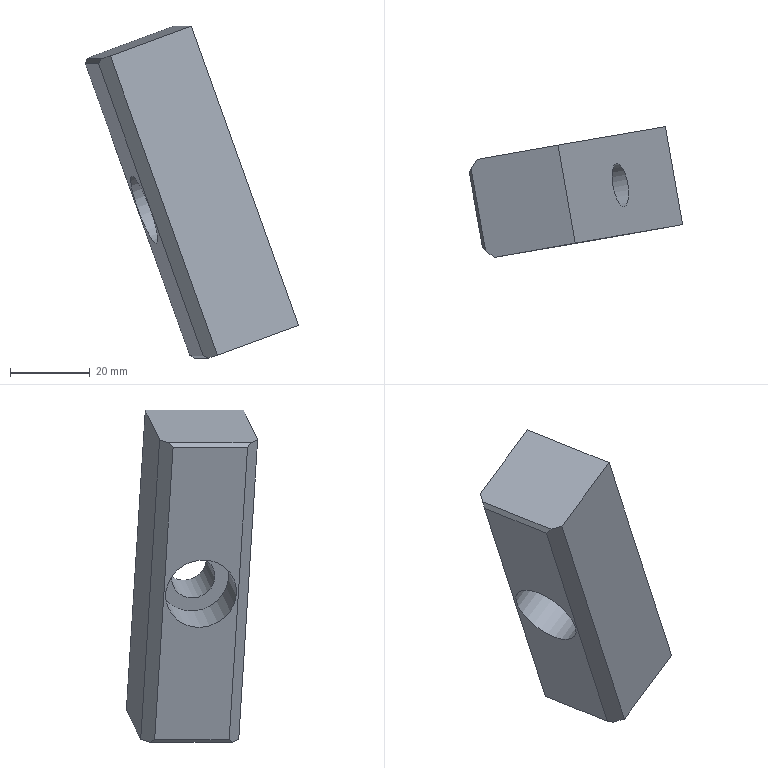Part | NX | features solid 2 | 1 solid | 13 faces | box 53.565 x 32.961 x 83.384 mm | volume 44971 mm3 | plane 11 | cylinder 2 | commonest cylinder face diameters 11 x1 18 x1
STEP:
#1=CARTESIAN_POINT('',(896.041,-33.81,-58.145));
#2=VERTEX_POINT('',#1);
#3=CARTESIAN_POINT('',(875.682,-37.399,-65.669));
#4=VERTEX_POINT('',#3);
#5=CARTESIAN_POINT('',(896.041,-33.81,-58.145));
#6=DIRECTION('',(-0.9254,-0.1632,-0.342));
#7=VECTOR('',#6,1000.);
#8=LINE('',#5,#7);
#9=EDGE_CURVE('',#2,#4,#8,.T.);
#10=ORIENTED_EDGE('',*,*,#9,.T.);
#11=CARTESIAN_POINT('',(902.628,-32.648,-140.845));
#12=VERTEX_POINT('',#11);
#13=CARTESIAN_POINT('',(875.682,-37.399,-65.669));
#14=DIRECTION('',(0.3368,0.05939,-0.9397));
#15=VECTOR('',#14,1000.);
#16=LINE('',#13,#15);
#17=EDGE_CURVE('',#4,#12,#16,.T.);
#18=ORIENTED_EDGE('',*,*,#17,.T.);
#19=CARTESIAN_POINT('',(922.987,-29.058,-133.32));
#20=VERTEX_POINT('',#19);
#21=CARTESIAN_POINT('',(922.987,-29.058,-133.32));
#22=DIRECTION('',(-0.9254,-0.1632,-0.342));
#23=VECTOR('',#22,1000.);
#24=LINE('',#21,#23);
#25=EDGE_CURVE('',#20,#12,#24,.T.);
#26=ORIENTED_EDGE('',*,*,#25,.F.);
#27=CARTESIAN_POINT('',(896.041,-33.81,-58.145));
#28=DIRECTION('',(0.3368,0.05939,-0.9397));
#29=VECTOR('',#28,1000.);
#30=LINE('',#27,#29);
#31=EDGE_CURVE('',#2,#20,#30,.T.);
#32=ORIENTED_EDGE('',*,*,#31,.F.);
#33=EDGE_LOOP('',(#10,#18,#26,#32));
#34=FACE_BOUND('',#33,.T.);
#35=CARTESIAN_POINT('',(896.041,-33.81,-58.145));
#36=DIRECTION('',(0.1736,-0.9848,0.));
#37=DIRECTION('',(-0.9254,-0.1632,-0.342));
#38=AXIS2_PLACEMENT_3D('',#35,#36,#37);
#39=PLANE('',#38);
#40=ADVANCED_FACE('',(#34),#39,.T.);
#41=CARTESIAN_POINT('',(887.328,-23.203,-112.725));
#42=VERTEX_POINT('',#41);
#43=CARTESIAN_POINT('',(884.208,-23.203,-104.283));
#44=DIRECTION('',(0.9254,0.1632,0.342));
#45=DIRECTION('',(0.3467,0.,-0.938));
#46=AXIS2_PLACEMENT_3D('',#43,#44,#45);
#47=CIRCLE('',#46,9.);
#48=EDGE_CURVE('',#42,#42,#47,.T.);
#49=ORIENTED_EDGE('',*,*,#48,.T.);
#50=EDGE_LOOP('',(#49));
#51=FACE_BOUND('',#50,.T.);
#52=CARTESIAN_POINT('',(898.994,-30.243,-140.931));
#53=VERTEX_POINT('',#52);
#54=CARTESIAN_POINT('',(872.721,-34.875,-67.635));
#55=VERTEX_POINT('',#54);
#56=CARTESIAN_POINT('',(872.385,-34.934,-66.695));
#57=DIRECTION('',(-0.3368,-0.05939,0.9397));
#58=VECTOR('',#57,1000.);
#59=LINE('',#56,#58);
#60=EDGE_CURVE('',#53,#55,#59,.T.);
#61=ORIENTED_EDGE('',*,*,#60,.T.);
#62=CARTESIAN_POINT('',(869.422,-16.164,-67.635));
#63=VERTEX_POINT('',#62);
#64=CARTESIAN_POINT('',(868.814,-12.717,-67.635));
#65=DIRECTION('',(-0.1736,0.9848,0.));
#66=VECTOR('',#65,1000.);
#67=LINE('',#64,#66);
#68=EDGE_CURVE('',#55,#63,#67,.T.);
#69=ORIENTED_EDGE('',*,*,#68,.T.);
#70=CARTESIAN_POINT('',(895.694,-11.531,-140.931));
#71=VERTEX_POINT('',#70);
#72=CARTESIAN_POINT('',(869.085,-16.223,-66.695));
#73=DIRECTION('',(0.3368,0.05939,-0.9397));
#74=VECTOR('',#73,1000.);
#75=LINE('',#72,#74);
#76=EDGE_CURVE('',#63,#71,#75,.T.);
#77=ORIENTED_EDGE('',*,*,#76,.T.);
#78=CARTESIAN_POINT('',(900.122,-36.644,-140.931));
#79=DIRECTION('',(0.1736,-0.9848,0.));
#80=VECTOR('',#79,1000.);
#81=LINE('',#78,#80);
#82=EDGE_CURVE('',#71,#53,#81,.T.);
#83=ORIENTED_EDGE('',*,*,#82,.T.);
#84=EDGE_LOOP('',(#61,#69,#77,#83));
#85=FACE_BOUND('',#84,.T.);
#86=CARTESIAN_POINT('',(873.513,-41.336,-66.695));
#87=DIRECTION('',(-0.9254,-0.1632,-0.342));
#88=DIRECTION('',(-0.1736,0.9848,0.));
#89=AXIS2_PLACEMENT_3D('',#86,#87,#88);
#90=PLANE('',#89);
#91=ADVANCED_FACE('',(#51,#85),#90,.T.);
#92=CARTESIAN_POINT('',(918.646,-4.438,-133.32));
#93=VERTEX_POINT('',#92);
#94=CARTESIAN_POINT('',(898.286,-8.028,-140.845));
#95=VERTEX_POINT('',#94);
#96=CARTESIAN_POINT('',(918.646,-4.438,-133.32));
#97=DIRECTION('',(0.9254,0.1632,0.342));
#98=VECTOR('',#97,1000.);
#99=LINE('',#96,#98);
#100=EDGE_CURVE('',#93,#95,#99,.F.);
#101=ORIENTED_EDGE('',*,*,#100,.T.);
#102=CARTESIAN_POINT('',(871.341,-12.779,-65.669));
#103=VERTEX_POINT('',#102);
#104=CARTESIAN_POINT('',(871.341,-12.779,-65.669));
#105=DIRECTION('',(0.3368,0.05939,-0.9397));
#106=VECTOR('',#105,1000.);
#107=LINE('',#104,#106);
#108=EDGE_CURVE('',#95,#103,#107,.F.);
#109=ORIENTED_EDGE('',*,*,#108,.T.);
#110=CARTESIAN_POINT('',(891.7,-9.189,-58.145));
#111=VERTEX_POINT('',#110);
#112=CARTESIAN_POINT('',(891.7,-9.189,-58.145));
#113=DIRECTION('',(0.9254,0.1632,0.342));
#114=VECTOR('',#113,1000.);
#115=LINE('',#112,#114);
#116=EDGE_CURVE('',#111,#103,#115,.F.);
#117=ORIENTED_EDGE('',*,*,#116,.F.);
#118=CARTESIAN_POINT('',(891.7,-9.189,-58.145));
#119=DIRECTION('',(0.3368,0.05939,-0.9397));
#120=VECTOR('',#119,1000.);
#121=LINE('',#118,#120);
#122=EDGE_CURVE('',#111,#93,#121,.T.);
#123=ORIENTED_EDGE('',*,*,#122,.T.);
#124=EDGE_LOOP('',(#101,#109,#117,#123));
#125=FACE_BOUND('',#124,.T.);
#126=CARTESIAN_POINT('',(891.7,-9.189,-58.145));
#127=DIRECTION('',(0.1736,-0.9848,0.));
#128=DIRECTION('',(-0.9254,-0.1632,-0.342));
#129=AXIS2_PLACEMENT_3D('',#126,#127,#128);
#130=PLANE('',#129);
#131=ADVANCED_FACE('',(#125),#130,.F.);
#132=CARTESIAN_POINT('',(905.437,-19.124,-90.574));
#133=VERTEX_POINT('',#132);
#134=CARTESIAN_POINT('',(907.343,-19.124,-95.733));
#135=DIRECTION('',(-0.9254,-0.1632,-0.342));
#136=DIRECTION('',(-0.3467,0.,0.938));
#137=AXIS2_PLACEMENT_3D('',#134,#135,#136);
#138=CIRCLE('',#137,5.5);
#139=EDGE_CURVE('',#133,#133,#138,.F.);
#140=ORIENTED_EDGE('',*,*,#139,.F.);
#141=EDGE_LOOP('',(#140));
#142=FACE_BOUND('',#141,.T.);
#143=CARTESIAN_POINT('',(896.649,-37.256,-58.145));
#144=DIRECTION('',(-0.1736,0.9848,0.));
#145=VECTOR('',#144,1000.);
#146=LINE('',#143,#145);
#147=EDGE_CURVE('',#2,#111,#146,.T.);
#148=ORIENTED_EDGE('',*,*,#147,.F.);
#149=ORIENTED_EDGE('',*,*,#31,.T.);
#150=CARTESIAN_POINT('',(923.595,-32.505,-133.32));
#151=DIRECTION('',(-0.1736,0.9848,0.));
#152=VECTOR('',#151,1000.);
#153=LINE('',#150,#152);
#154=EDGE_CURVE('',#20,#93,#153,.T.);
#155=ORIENTED_EDGE('',*,*,#154,.T.);
#156=ORIENTED_EDGE('',*,*,#122,.F.);
#157=EDGE_LOOP('',(#148,#149,#155,#156));
#158=FACE_BOUND('',#157,.T.);
#159=CARTESIAN_POINT('',(896.649,-37.256,-58.145));
#160=DIRECTION('',(-0.9254,-0.1632,-0.342));
#161=DIRECTION('',(-0.1736,0.9848,0.));
#162=AXIS2_PLACEMENT_3D('',#159,#160,#161);
#163=PLANE('',#162);
#164=ADVANCED_FACE('',(#142,#158),#163,.F.);
#165=CARTESIAN_POINT('',(900.43,-31.005,-141.529));
#166=VERTEX_POINT('',#165);
#167=CARTESIAN_POINT('',(917.465,-43.74,-136.228));
#168=DIRECTION('',(0.7772,-0.581,0.2418));
#169=VECTOR('',#168,1000.);
#170=LINE('',#167,#169);
#171=EDGE_CURVE('',#12,#166,#170,.F.);
#172=ORIENTED_EDGE('',*,*,#171,.T.);
#173=CARTESIAN_POINT('',(896.783,-10.324,-141.529));
#174=VERTEX_POINT('',#173);
#175=CARTESIAN_POINT('',(901.385,-36.421,-141.529));
#176=DIRECTION('',(-0.1736,0.9848,0.));
#177=VECTOR('',#176,1000.);
#178=LINE('',#175,#177);
#179=EDGE_CURVE('',#166,#174,#178,.T.);
#180=ORIENTED_EDGE('',*,*,#179,.T.);
#181=CARTESIAN_POINT('',(896.407,-10.898,-141.7));
#182=DIRECTION('',(0.5316,0.8117,0.2418));
#183=VECTOR('',#182,1000.);
#184=LINE('',#181,#183);
#185=EDGE_CURVE('',#174,#95,#184,.T.);
#186=ORIENTED_EDGE('',*,*,#185,.T.);
#187=ORIENTED_EDGE('',*,*,#100,.F.);
#188=ORIENTED_EDGE('',*,*,#154,.F.);
#189=ORIENTED_EDGE('',*,*,#25,.T.);
#190=EDGE_LOOP('',(#172,#180,#186,#187,#188,#189));
#191=FACE_BOUND('',#190,.T.);
#192=CARTESIAN_POINT('',(923.595,-32.505,-133.32));
#193=DIRECTION('',(0.3368,0.05939,-0.9397));
#194=DIRECTION('',(-0.9414,0.,-0.3374));
#195=AXIS2_PLACEMENT_3D('',#192,#193,#194);
#196=PLANE('',#195);
#197=ADVANCED_FACE('',(#191),#196,.T.);
#198=CARTESIAN_POINT('',(869.837,-15.075,-66.353));
#199=VERTEX_POINT('',#198);
#200=CARTESIAN_POINT('',(869.085,-16.223,-66.695));
#201=DIRECTION('',(-0.5316,-0.8117,-0.2418));
#202=VECTOR('',#201,1000.);
#203=LINE('',#200,#202);
#204=EDGE_CURVE('',#103,#199,#203,.T.);
#205=ORIENTED_EDGE('',*,*,#204,.T.);
#206=CARTESIAN_POINT('',(873.484,-35.756,-66.353));
#207=VERTEX_POINT('',#206);
#208=CARTESIAN_POINT('',(873.918,-38.218,-66.353));
#209=DIRECTION('',(0.1736,-0.9848,0.));
#210=VECTOR('',#209,1000.);
#211=LINE('',#208,#210);
#212=EDGE_CURVE('',#199,#207,#211,.T.);
#213=ORIENTED_EDGE('',*,*,#212,.T.);
#214=CARTESIAN_POINT('',(875.682,-37.399,-65.669));
#215=DIRECTION('',(-0.7772,0.581,-0.2418));
#216=VECTOR('',#215,1000.);
#217=LINE('',#214,#216);
#218=EDGE_CURVE('',#207,#4,#217,.F.);
#219=ORIENTED_EDGE('',*,*,#218,.T.);
#220=ORIENTED_EDGE('',*,*,#9,.F.);
#221=ORIENTED_EDGE('',*,*,#147,.T.);
#222=ORIENTED_EDGE('',*,*,#116,.T.);
#223=EDGE_LOOP('',(#205,#213,#219,#220,#221,#222));
#224=FACE_BOUND('',#223,.T.);
#225=CARTESIAN_POINT('',(896.649,-37.256,-58.145));
#226=DIRECTION('',(0.3368,0.05939,-0.9397));
#227=DIRECTION('',(-0.9414,0.,-0.3374));
#228=AXIS2_PLACEMENT_3D('',#225,#226,#227);
#229=PLANE('',#228);
#230=ADVANCED_FACE('',(#224),#229,.F.);
#231=ORIENTED_EDGE('',*,*,#76,.F.);
#232=CARTESIAN_POINT('',(869.56,-15.801,-67.208));
#233=DIRECTION('',(0.2396,0.6285,0.74));
#234=VECTOR('',#233,1000.);
#235=LINE('',#232,#234);
#236=EDGE_CURVE('',#63,#199,#235,.T.);
#237=ORIENTED_EDGE('',*,*,#236,.T.);
#238=ORIENTED_EDGE('',*,*,#204,.F.);
#239=ORIENTED_EDGE('',*,*,#108,.F.);
#240=ORIENTED_EDGE('',*,*,#185,.F.);
#241=CARTESIAN_POINT('',(867.028,-43.325,-125.192));
#242=DIRECTION('',(0.6285,0.6971,-0.3451));
#243=VECTOR('',#242,1000.);
#244=LINE('',#241,#243);
#245=EDGE_CURVE('',#174,#71,#244,.F.);
#246=ORIENTED_EDGE('',*,*,#245,.T.);
#247=EDGE_LOOP('',(#231,#237,#238,#239,#240,#246));
#248=FACE_BOUND('',#247,.T.);
#249=CARTESIAN_POINT('',(869.085,-16.223,-66.695));
#250=DIRECTION('',(-0.7772,0.581,-0.2418));
#251=DIRECTION('',(-0.5988,-0.8009,0.));
#252=AXIS2_PLACEMENT_3D('',#249,#250,#251);
#253=PLANE('',#252);
#254=ADVANCED_FACE('',(#248),#253,.T.);
#255=ORIENTED_EDGE('',*,*,#218,.F.);
#256=CARTESIAN_POINT('',(874.5,-36.931,-64.644));
#257=DIRECTION('',(0.4401,-0.5087,0.74));
#258=VECTOR('',#257,1000.);
#259=LINE('',#256,#258);
#260=EDGE_CURVE('',#207,#55,#259,.F.);
#261=ORIENTED_EDGE('',*,*,#260,.T.);
#262=ORIENTED_EDGE('',*,*,#60,.F.);
#263=CARTESIAN_POINT('',(864.054,-11.695,-126.388));
#264=DIRECTION('',(0.829,-0.4401,-0.3451));
#265=VECTOR('',#264,1000.);
#266=LINE('',#263,#265);
#267=EDGE_CURVE('',#53,#166,#266,.T.);
#268=ORIENTED_EDGE('',*,*,#267,.T.);
#269=ORIENTED_EDGE('',*,*,#171,.F.);
#270=ORIENTED_EDGE('',*,*,#17,.F.);
#271=EDGE_LOOP('',(#255,#261,#262,#268,#269,#270));
#272=FACE_BOUND('',#271,.T.);
#273=CARTESIAN_POINT('',(875.682,-37.399,-65.669));
#274=DIRECTION('',(0.5316,0.8117,0.2418));
#275=DIRECTION('',(-0.8366,0.5478,0.));
#276=AXIS2_PLACEMENT_3D('',#273,#274,#275);
#277=PLANE('',#276);
#278=ADVANCED_FACE('',(#272),#277,.F.);
#279=ORIENTED_EDGE('',*,*,#260,.F.);
#280=ORIENTED_EDGE('',*,*,#212,.F.);
#281=ORIENTED_EDGE('',*,*,#236,.F.);
#282=ORIENTED_EDGE('',*,*,#68,.F.);
#283=EDGE_LOOP('',(#279,#280,#281,#282));
#284=FACE_BOUND('',#283,.T.);
#285=CARTESIAN_POINT('',(873.85,-41.276,-67.635));
#286=DIRECTION('',(-0.8925,-0.1574,0.4226));
#287=DIRECTION('',(0.428,0.,0.9038));
#288=AXIS2_PLACEMENT_3D('',#285,#286,#287);
#289=PLANE('',#288);
#290=ADVANCED_FACE('',(#284),#289,.T.);
#291=ORIENTED_EDGE('',*,*,#267,.F.);
#292=ORIENTED_EDGE('',*,*,#82,.F.);
#293=ORIENTED_EDGE('',*,*,#245,.F.);
#294=ORIENTED_EDGE('',*,*,#179,.F.);
#295=EDGE_LOOP('',(#291,#292,#293,#294));
#296=FACE_BOUND('',#295,.T.);
#297=CARTESIAN_POINT('',(901.385,-36.421,-141.529));
#298=DIRECTION('',(0.4162,0.07339,0.9063));
#299=DIRECTION('',(0.9088,0.,-0.4173));
#300=AXIS2_PLACEMENT_3D('',#297,#298,#299);
#301=PLANE('',#300);
#302=ADVANCED_FACE('',(#296),#301,.F.);
#303=ORIENTED_EDGE('',*,*,#139,.T.);
#304=EDGE_LOOP('',(#303));
#305=FACE_BOUND('',#304,.T.);
#306=CARTESIAN_POINT('',(897.22,-21.245,-105.338));
#307=VERTEX_POINT('',#306);
#308=CARTESIAN_POINT('',(895.313,-21.245,-100.179));
#309=DIRECTION('',(0.9254,0.1632,0.342));
#310=DIRECTION('',(0.3467,0.,-0.938));
#311=AXIS2_PLACEMENT_3D('',#308,#309,#310);
#312=CIRCLE('',#311,5.5);
#313=EDGE_CURVE('',#307,#307,#312,.T.);
#314=ORIENTED_EDGE('',*,*,#313,.F.);
#315=EDGE_LOOP('',(#314));
#316=FACE_BOUND('',#315,.T.);
#317=CARTESIAN_POINT('',(972.122,-7.701,-71.791));
#318=DIRECTION('',(0.9254,0.1632,0.342));
#319=DIRECTION('',(0.3467,0.,-0.938));
#320=AXIS2_PLACEMENT_3D('',#317,#318,#319);
#321=CYLINDRICAL_SURFACE('',#320,5.5);
#322=ADVANCED_FACE('',(#305,#316),#321,.F.);
#323=ORIENTED_EDGE('',*,*,#313,.T.);
#324=EDGE_LOOP('',(#323));
#325=FACE_BOUND('',#324,.T.);
#326=CARTESIAN_POINT('',(898.433,-21.245,-108.621));
#327=VERTEX_POINT('',#326);
#328=CARTESIAN_POINT('',(895.313,-21.245,-100.179));
#329=DIRECTION('',(0.9254,0.1632,0.342));
#330=DIRECTION('',(0.3467,0.,-0.938));
#331=AXIS2_PLACEMENT_3D('',#328,#329,#330);
#332=CIRCLE('',#331,9.);
#333=EDGE_CURVE('',#327,#327,#332,.T.);
#334=ORIENTED_EDGE('',*,*,#333,.F.);
#335=EDGE_LOOP('',(#334));
#336=FACE_BOUND('',#335,.T.);
#337=CARTESIAN_POINT('',(895.313,-21.245,-100.179));
#338=DIRECTION('',(0.9254,0.1632,0.342));
#339=DIRECTION('',(0.3467,0.,-0.938));
#340=AXIS2_PLACEMENT_3D('',#337,#338,#339);
#341=PLANE('',#340);
#342=ADVANCED_FACE('',(#325,#336),#341,.F.);
#343=ORIENTED_EDGE('',*,*,#333,.T.);
#344=EDGE_LOOP('',(#343));
#345=FACE_BOUND('',#344,.T.);
#346=ORIENTED_EDGE('',*,*,#48,.F.);
#347=EDGE_LOOP('',(#346));
#348=FACE_BOUND('',#347,.T.);
#349=CARTESIAN_POINT('',(884.208,-23.203,-104.283));
#350=DIRECTION('',(0.9254,0.1632,0.342));
#351=DIRECTION('',(0.3467,0.,-0.938));
#352=AXIS2_PLACEMENT_3D('',#349,#350,#351);
#353=CYLINDRICAL_SURFACE('',#352,9.);
#354=ADVANCED_FACE('',(#345,#348),#353,.F.);
#355=CLOSED_SHELL('',(#40,#91,#131,#164,#197,#230,#254,#278,#290,#302,#322,#342,#354));
#356=MANIFOLD_SOLID_BREP('',#355);
#357=(LENGTH_UNIT()NAMED_UNIT(*)SI_UNIT(.MILLI.,.METRE.));
#358=UNCERTAINTY_MEASURE_WITH_UNIT(LENGTH_MEASURE(0.00001),#357,'','');
#359=(NAMED_UNIT(*)PLANE_ANGLE_UNIT()SI_UNIT($,.RADIAN.));
#360=(NAMED_UNIT(*)SI_UNIT($,.STERADIAN.)SOLID_ANGLE_UNIT());
#361=(GEOMETRIC_REPRESENTATION_CONTEXT(3)GLOBAL_UNCERTAINTY_ASSIGNED_CONTEXT((#358))GLOBAL_UNIT_ASSIGNED_CONTEXT((#357,#359,#360))REPRESENTATION_CONTEXT('',''));
#362=ADVANCED_BREP_SHAPE_REPRESENTATION('',(#356),#361);